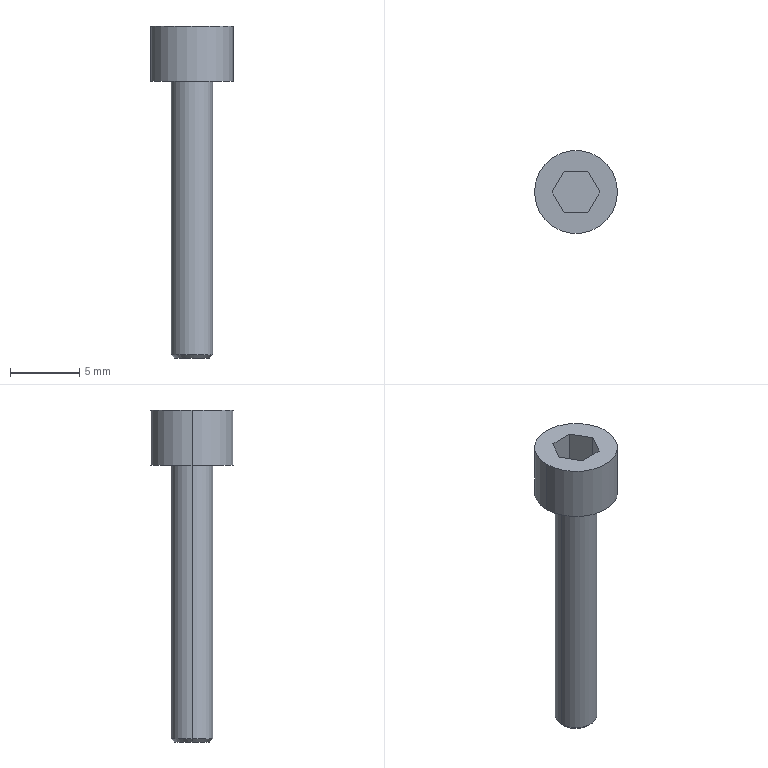Part | SolidWorks | features BaseBody 1 | 1 solid | 16 faces | box 6 x 6 x 24 mm | volume 234.705 mm3 | plane 10 | cylinder 4 | cone 2 | commonest cylinder face diameters 3 x2 6 x2
STEP:
#1=CARTESIAN_POINT('',(1.25,0.,-20.));
#2=VERTEX_POINT('',#1);
#3=CARTESIAN_POINT('',(-1.25,0.,-20.));
#4=VERTEX_POINT('',#3);
#5=CARTESIAN_POINT('',(0.,0.,-20.));
#6=DIRECTION('',(0.,0.,1.));
#7=DIRECTION('',(1.,0.,0.));
#8=AXIS2_PLACEMENT_3D('',#5,#6,#7);
#9=CIRCLE('',#8,1.25);
#10=EDGE_CURVE('',#2,#4,#9,.T.);
#11=ORIENTED_EDGE('',*,*,#10,.T.);
#12=CARTESIAN_POINT('',(-1.5,0.,-19.75));
#13=VERTEX_POINT('',#12);
#14=CARTESIAN_POINT('',(-1.375,0.,-19.875));
#15=DIRECTION('',(-0.7071,0.,0.7071));
#16=VECTOR('',#15,1000.);
#17=LINE('',#14,#16);
#18=EDGE_CURVE('',#4,#13,#17,.T.);
#19=ORIENTED_EDGE('',*,*,#18,.T.);
#20=CARTESIAN_POINT('',(1.5,0.,-19.75));
#21=VERTEX_POINT('',#20);
#22=CARTESIAN_POINT('',(0.,0.,-19.75));
#23=DIRECTION('',(0.,0.,-1.));
#24=DIRECTION('',(1.,0.,0.));
#25=AXIS2_PLACEMENT_3D('',#22,#23,#24);
#26=CIRCLE('',#25,1.5);
#27=EDGE_CURVE('',#13,#21,#26,.T.);
#28=ORIENTED_EDGE('',*,*,#27,.T.);
#29=CARTESIAN_POINT('',(1.375,0.,-19.875));
#30=DIRECTION('',(0.7071,0.,0.7071));
#31=VECTOR('',#30,1000.);
#32=LINE('',#29,#31);
#33=EDGE_CURVE('',#2,#21,#32,.T.);
#34=ORIENTED_EDGE('',*,*,#33,.F.);
#35=EDGE_LOOP('',(#11,#19,#28,#34));
#36=FACE_OUTER_BOUND('',#35,.T.);
#37=CARTESIAN_POINT('',(0.,0.,-19.875));
#38=DIRECTION('',(0.,0.,1.));
#39=DIRECTION('',(1.,0.,0.));
#40=AXIS2_PLACEMENT_3D('',#37,#38,#39);
#41=CONICAL_SURFACE('',#40,1.375,0.7854);
#42=ADVANCED_FACE('',(#36),#41,.T.);
#43=ORIENTED_EDGE('',*,*,#27,.F.);
#44=CARTESIAN_POINT('',(-1.5,0.,0.));
#45=VERTEX_POINT('',#44);
#46=CARTESIAN_POINT('',(-1.5,0.,0.));
#47=DIRECTION('',(0.,0.,1.));
#48=VECTOR('',#47,1000.);
#49=LINE('',#46,#48);
#50=EDGE_CURVE('',#13,#45,#49,.T.);
#51=ORIENTED_EDGE('',*,*,#50,.T.);
#52=CARTESIAN_POINT('',(1.5,0.,0.));
#53=VERTEX_POINT('',#52);
#54=CARTESIAN_POINT('',(0.,0.,0.));
#55=DIRECTION('',(0.,0.,1.));
#56=DIRECTION('',(1.,0.,0.));
#57=AXIS2_PLACEMENT_3D('',#54,#55,#56);
#58=CIRCLE('',#57,1.5);
#59=EDGE_CURVE('',#53,#45,#58,.T.);
#60=ORIENTED_EDGE('',*,*,#59,.F.);
#61=CARTESIAN_POINT('',(1.5,0.,0.));
#62=DIRECTION('',(0.,0.,1.));
#63=VECTOR('',#62,1000.);
#64=LINE('',#61,#63);
#65=EDGE_CURVE('',#21,#53,#64,.T.);
#66=ORIENTED_EDGE('',*,*,#65,.F.);
#67=EDGE_LOOP('',(#43,#51,#60,#66));
#68=FACE_OUTER_BOUND('',#67,.T.);
#69=CARTESIAN_POINT('',(0.,0.,0.));
#70=DIRECTION('',(0.,0.,1.));
#71=DIRECTION('',(1.,0.,0.));
#72=AXIS2_PLACEMENT_3D('',#69,#70,#71);
#73=CYLINDRICAL_SURFACE('',#72,1.5);
#74=ADVANCED_FACE('',(#68),#73,.T.);
#75=CARTESIAN_POINT('',(3.,0.,4.));
#76=VERTEX_POINT('',#75);
#77=CARTESIAN_POINT('',(-3.,0.,4.));
#78=VERTEX_POINT('',#77);
#79=CARTESIAN_POINT('',(0.,0.,4.));
#80=DIRECTION('',(0.,0.,1.));
#81=DIRECTION('',(-1.,0.,0.));
#82=AXIS2_PLACEMENT_3D('',#79,#80,#81);
#83=CIRCLE('',#82,3.);
#84=EDGE_CURVE('',#76,#78,#83,.T.);
#85=ORIENTED_EDGE('',*,*,#84,.F.);
#86=CARTESIAN_POINT('',(3.,0.,0.));
#87=VERTEX_POINT('',#86);
#88=CARTESIAN_POINT('',(3.,0.,0.));
#89=DIRECTION('',(0.,0.,-1.));
#90=VECTOR('',#89,1000.);
#91=LINE('',#88,#90);
#92=EDGE_CURVE('',#76,#87,#91,.T.);
#93=ORIENTED_EDGE('',*,*,#92,.T.);
#94=CARTESIAN_POINT('',(-3.,0.,0.));
#95=VERTEX_POINT('',#94);
#96=CARTESIAN_POINT('',(0.,0.,0.));
#97=DIRECTION('',(0.,0.,-1.));
#98=DIRECTION('',(-1.,0.,0.));
#99=AXIS2_PLACEMENT_3D('',#96,#97,#98);
#100=CIRCLE('',#99,3.);
#101=EDGE_CURVE('',#95,#87,#100,.T.);
#102=ORIENTED_EDGE('',*,*,#101,.F.);
#103=CARTESIAN_POINT('',(-3.,0.,0.));
#104=DIRECTION('',(0.,0.,-1.));
#105=VECTOR('',#104,1000.);
#106=LINE('',#103,#105);
#107=EDGE_CURVE('',#78,#95,#106,.T.);
#108=ORIENTED_EDGE('',*,*,#107,.F.);
#109=EDGE_LOOP('',(#85,#93,#102,#108));
#110=FACE_OUTER_BOUND('',#109,.T.);
#111=CARTESIAN_POINT('',(0.,0.,0.));
#112=DIRECTION('',(0.,0.,-1.));
#113=DIRECTION('',(-1.,0.,0.));
#114=AXIS2_PLACEMENT_3D('',#111,#112,#113);
#115=CYLINDRICAL_SURFACE('',#114,3.);
#116=ADVANCED_FACE('',(#110),#115,.T.);
#117=ORIENTED_EDGE('',*,*,#10,.F.);
#118=CARTESIAN_POINT('',(0.,0.,-20.));
#119=DIRECTION('',(0.,0.,1.));
#120=DIRECTION('',(1.,0.,0.));
#121=AXIS2_PLACEMENT_3D('',#118,#119,#120);
#122=CIRCLE('',#121,1.25);
#123=EDGE_CURVE('',#4,#2,#122,.T.);
#124=ORIENTED_EDGE('',*,*,#123,.F.);
#125=EDGE_LOOP('',(#117,#124));
#126=FACE_OUTER_BOUND('',#125,.T.);
#127=CARTESIAN_POINT('',(0.,0.,-20.));
#128=DIRECTION('',(0.,0.,1.));
#129=DIRECTION('',(1.,0.,0.));
#130=AXIS2_PLACEMENT_3D('',#127,#128,#129);
#131=PLANE('',#130);
#132=ADVANCED_FACE('',(#126),#131,.F.);
#133=CARTESIAN_POINT('',(1.732,0.,4.));
#134=VERTEX_POINT('',#133);
#135=CARTESIAN_POINT('',(0.866,-1.5,4.));
#136=VERTEX_POINT('',#135);
#137=CARTESIAN_POINT('',(1.516,-0.375,4.));
#138=DIRECTION('',(-0.5,-0.866,0.));
#139=VECTOR('',#138,1000.);
#140=LINE('',#137,#139);
#141=EDGE_CURVE('',#134,#136,#140,.T.);
#142=ORIENTED_EDGE('',*,*,#141,.F.);
#143=CARTESIAN_POINT('',(1.732,0.,1.5));
#144=VERTEX_POINT('',#143);
#145=CARTESIAN_POINT('',(1.732,0.,4.));
#146=DIRECTION('',(0.,0.,-1.));
#147=VECTOR('',#146,1000.);
#148=LINE('',#145,#147);
#149=EDGE_CURVE('',#134,#144,#148,.T.);
#150=ORIENTED_EDGE('',*,*,#149,.T.);
#151=CARTESIAN_POINT('',(0.866,-1.5,1.5));
#152=VERTEX_POINT('',#151);
#153=CARTESIAN_POINT('',(1.732,0.,1.5));
#154=DIRECTION('',(-0.5,-0.866,0.));
#155=VECTOR('',#154,1000.);
#156=LINE('',#153,#155);
#157=EDGE_CURVE('',#144,#152,#156,.T.);
#158=ORIENTED_EDGE('',*,*,#157,.T.);
#159=CARTESIAN_POINT('',(0.866,-1.5,4.));
#160=DIRECTION('',(0.,0.,-1.));
#161=VECTOR('',#160,1000.);
#162=LINE('',#159,#161);
#163=EDGE_CURVE('',#136,#152,#162,.T.);
#164=ORIENTED_EDGE('',*,*,#163,.F.);
#165=EDGE_LOOP('',(#142,#150,#158,#164));
#166=FACE_OUTER_BOUND('',#165,.T.);
#167=CARTESIAN_POINT('',(1.732,0.,4.));
#168=DIRECTION('',(0.866,-0.5,0.));
#169=DIRECTION('',(0.,0.,-1.));
#170=AXIS2_PLACEMENT_3D('',#167,#168,#169);
#171=PLANE('',#170);
#172=ADVANCED_FACE('',(#166),#171,.F.);
#173=CARTESIAN_POINT('',(0.866,1.5,4.));
#174=VERTEX_POINT('',#173);
#175=CARTESIAN_POINT('',(1.083,1.125,4.));
#176=DIRECTION('',(0.5,-0.866,0.));
#177=VECTOR('',#176,1000.);
#178=LINE('',#175,#177);
#179=EDGE_CURVE('',#174,#134,#178,.T.);
#180=ORIENTED_EDGE('',*,*,#179,.F.);
#181=CARTESIAN_POINT('',(0.866,1.5,1.5));
#182=VERTEX_POINT('',#181);
#183=CARTESIAN_POINT('',(0.866,1.5,4.));
#184=DIRECTION('',(0.,0.,-1.));
#185=VECTOR('',#184,1000.);
#186=LINE('',#183,#185);
#187=EDGE_CURVE('',#174,#182,#186,.T.);
#188=ORIENTED_EDGE('',*,*,#187,.T.);
#189=CARTESIAN_POINT('',(0.866,1.5,1.5));
#190=DIRECTION('',(0.5,-0.866,0.));
#191=VECTOR('',#190,1000.);
#192=LINE('',#189,#191);
#193=EDGE_CURVE('',#182,#144,#192,.T.);
#194=ORIENTED_EDGE('',*,*,#193,.T.);
#195=ORIENTED_EDGE('',*,*,#149,.F.);
#196=EDGE_LOOP('',(#180,#188,#194,#195));
#197=FACE_OUTER_BOUND('',#196,.T.);
#198=CARTESIAN_POINT('',(0.866,1.5,4.));
#199=DIRECTION('',(0.866,0.5,0.));
#200=DIRECTION('',(0.,0.,-1.));
#201=AXIS2_PLACEMENT_3D('',#198,#199,#200);
#202=PLANE('',#201);
#203=ADVANCED_FACE('',(#197),#202,.F.);
#204=CARTESIAN_POINT('',(-0.866,1.5,4.));
#205=VERTEX_POINT('',#204);
#206=CARTESIAN_POINT('',(-0.433,1.5,4.));
#207=DIRECTION('',(1.,0.,0.));
#208=VECTOR('',#207,1000.);
#209=LINE('',#206,#208);
#210=EDGE_CURVE('',#205,#174,#209,.T.);
#211=ORIENTED_EDGE('',*,*,#210,.F.);
#212=CARTESIAN_POINT('',(-0.866,1.5,1.5));
#213=VERTEX_POINT('',#212);
#214=CARTESIAN_POINT('',(-0.866,1.5,4.));
#215=DIRECTION('',(0.,0.,-1.));
#216=VECTOR('',#215,1000.);
#217=LINE('',#214,#216);
#218=EDGE_CURVE('',#205,#213,#217,.T.);
#219=ORIENTED_EDGE('',*,*,#218,.T.);
#220=CARTESIAN_POINT('',(-0.866,1.5,1.5));
#221=DIRECTION('',(1.,0.,0.));
#222=VECTOR('',#221,1000.);
#223=LINE('',#220,#222);
#224=EDGE_CURVE('',#213,#182,#223,.T.);
#225=ORIENTED_EDGE('',*,*,#224,.T.);
#226=ORIENTED_EDGE('',*,*,#187,.F.);
#227=EDGE_LOOP('',(#211,#219,#225,#226));
#228=FACE_OUTER_BOUND('',#227,.T.);
#229=CARTESIAN_POINT('',(-0.866,1.5,4.));
#230=DIRECTION('',(0.,1.,0.));
#231=DIRECTION('',(1.,0.,0.));
#232=AXIS2_PLACEMENT_3D('',#229,#230,#231);
#233=PLANE('',#232);
#234=ADVANCED_FACE('',(#228),#233,.F.);
#235=CARTESIAN_POINT('',(-1.732,0.,4.));
#236=VERTEX_POINT('',#235);
#237=CARTESIAN_POINT('',(-1.516,0.375,4.));
#238=DIRECTION('',(0.5,0.866,0.));
#239=VECTOR('',#238,1000.);
#240=LINE('',#237,#239);
#241=EDGE_CURVE('',#236,#205,#240,.T.);
#242=ORIENTED_EDGE('',*,*,#241,.F.);
#243=CARTESIAN_POINT('',(-1.732,0.,1.5));
#244=VERTEX_POINT('',#243);
#245=CARTESIAN_POINT('',(-1.732,0.,4.));
#246=DIRECTION('',(0.,0.,-1.));
#247=VECTOR('',#246,1000.);
#248=LINE('',#245,#247);
#249=EDGE_CURVE('',#236,#244,#248,.T.);
#250=ORIENTED_EDGE('',*,*,#249,.T.);
#251=CARTESIAN_POINT('',(-1.732,0.,1.5));
#252=DIRECTION('',(0.5,0.866,0.));
#253=VECTOR('',#252,1000.);
#254=LINE('',#251,#253);
#255=EDGE_CURVE('',#244,#213,#254,.T.);
#256=ORIENTED_EDGE('',*,*,#255,.T.);
#257=ORIENTED_EDGE('',*,*,#218,.F.);
#258=EDGE_LOOP('',(#242,#250,#256,#257));
#259=FACE_OUTER_BOUND('',#258,.T.);
#260=CARTESIAN_POINT('',(-1.732,0.,4.));
#261=DIRECTION('',(-0.866,0.5,0.));
#262=DIRECTION('',(0.,0.,1.));
#263=AXIS2_PLACEMENT_3D('',#260,#261,#262);
#264=PLANE('',#263);
#265=ADVANCED_FACE('',(#259),#264,.F.);
#266=CARTESIAN_POINT('',(-0.866,-1.5,4.));
#267=VERTEX_POINT('',#266);
#268=CARTESIAN_POINT('',(-1.083,-1.125,4.));
#269=DIRECTION('',(-0.5,0.866,0.));
#270=VECTOR('',#269,1000.);
#271=LINE('',#268,#270);
#272=EDGE_CURVE('',#267,#236,#271,.T.);
#273=ORIENTED_EDGE('',*,*,#272,.F.);
#274=CARTESIAN_POINT('',(-0.866,-1.5,1.5));
#275=VERTEX_POINT('',#274);
#276=CARTESIAN_POINT('',(-0.866,-1.5,4.));
#277=DIRECTION('',(0.,0.,-1.));
#278=VECTOR('',#277,1000.);
#279=LINE('',#276,#278);
#280=EDGE_CURVE('',#267,#275,#279,.T.);
#281=ORIENTED_EDGE('',*,*,#280,.T.);
#282=CARTESIAN_POINT('',(-0.866,-1.5,1.5));
#283=DIRECTION('',(-0.5,0.866,0.));
#284=VECTOR('',#283,1000.);
#285=LINE('',#282,#284);
#286=EDGE_CURVE('',#275,#244,#285,.T.);
#287=ORIENTED_EDGE('',*,*,#286,.T.);
#288=ORIENTED_EDGE('',*,*,#249,.F.);
#289=EDGE_LOOP('',(#273,#281,#287,#288));
#290=FACE_OUTER_BOUND('',#289,.T.);
#291=CARTESIAN_POINT('',(-0.866,-1.5,4.));
#292=DIRECTION('',(-0.866,-0.5,0.));
#293=DIRECTION('',(-0.5,0.866,0.));
#294=AXIS2_PLACEMENT_3D('',#291,#292,#293);
#295=PLANE('',#294);
#296=ADVANCED_FACE('',(#290),#295,.F.);
#297=CARTESIAN_POINT('',(0.433,-1.5,4.));
#298=DIRECTION('',(-1.,0.,0.));
#299=VECTOR('',#298,1000.);
#300=LINE('',#297,#299);
#301=EDGE_CURVE('',#136,#267,#300,.T.);
#302=ORIENTED_EDGE('',*,*,#301,.F.);
#303=ORIENTED_EDGE('',*,*,#163,.T.);
#304=CARTESIAN_POINT('',(0.866,-1.5,1.5));
#305=DIRECTION('',(-1.,0.,0.));
#306=VECTOR('',#305,1000.);
#307=LINE('',#304,#306);
#308=EDGE_CURVE('',#152,#275,#307,.T.);
#309=ORIENTED_EDGE('',*,*,#308,.T.);
#310=ORIENTED_EDGE('',*,*,#280,.F.);
#311=EDGE_LOOP('',(#302,#303,#309,#310));
#312=FACE_OUTER_BOUND('',#311,.T.);
#313=CARTESIAN_POINT('',(0.866,-1.5,4.));
#314=DIRECTION('',(0.,-1.,0.));
#315=DIRECTION('',(-1.,0.,0.));
#316=AXIS2_PLACEMENT_3D('',#313,#314,#315);
#317=PLANE('',#316);
#318=ADVANCED_FACE('',(#312),#317,.F.);
#319=ORIENTED_EDGE('',*,*,#308,.F.);
#320=ORIENTED_EDGE('',*,*,#157,.F.);
#321=ORIENTED_EDGE('',*,*,#193,.F.);
#322=ORIENTED_EDGE('',*,*,#224,.F.);
#323=ORIENTED_EDGE('',*,*,#255,.F.);
#324=ORIENTED_EDGE('',*,*,#286,.F.);
#325=EDGE_LOOP('',(#319,#320,#321,#322,#323,#324));
#326=FACE_OUTER_BOUND('',#325,.T.);
#327=CARTESIAN_POINT('',(0.,0.,1.5));
#328=DIRECTION('',(0.,0.,-1.));
#329=DIRECTION('',(0.,-1.,0.));
#330=AXIS2_PLACEMENT_3D('',#327,#328,#329);
#331=PLANE('',#330);
#332=ADVANCED_FACE('',(#326),#331,.F.);
#333=ORIENTED_EDGE('',*,*,#59,.T.);
#334=CARTESIAN_POINT('',(0.,0.,0.));
#335=DIRECTION('',(0.,0.,1.));
#336=DIRECTION('',(1.,0.,0.));
#337=AXIS2_PLACEMENT_3D('',#334,#335,#336);
#338=CIRCLE('',#337,1.5);
#339=EDGE_CURVE('',#45,#53,#338,.T.);
#340=ORIENTED_EDGE('',*,*,#339,.T.);
#341=EDGE_LOOP('',(#333,#340));
#342=FACE_BOUND('',#341,.T.);
#343=ORIENTED_EDGE('',*,*,#101,.T.);
#344=CARTESIAN_POINT('',(0.,0.,0.));
#345=DIRECTION('',(0.,0.,-1.));
#346=DIRECTION('',(-1.,0.,0.));
#347=AXIS2_PLACEMENT_3D('',#344,#345,#346);
#348=CIRCLE('',#347,3.);
#349=EDGE_CURVE('',#87,#95,#348,.T.);
#350=ORIENTED_EDGE('',*,*,#349,.T.);
#351=EDGE_LOOP('',(#343,#350));
#352=FACE_OUTER_BOUND('',#351,.T.);
#353=CARTESIAN_POINT('',(0.,0.,0.));
#354=DIRECTION('',(0.,0.,1.));
#355=DIRECTION('',(1.,0.,0.));
#356=AXIS2_PLACEMENT_3D('',#353,#354,#355);
#357=PLANE('',#356);
#358=ADVANCED_FACE('',(#342,#352),#357,.F.);
#359=ORIENTED_EDGE('',*,*,#141,.T.);
#360=ORIENTED_EDGE('',*,*,#301,.T.);
#361=ORIENTED_EDGE('',*,*,#272,.T.);
#362=ORIENTED_EDGE('',*,*,#241,.T.);
#363=ORIENTED_EDGE('',*,*,#210,.T.);
#364=ORIENTED_EDGE('',*,*,#179,.T.);
#365=EDGE_LOOP('',(#359,#360,#361,#362,#363,#364));
#366=FACE_BOUND('',#365,.T.);
#367=CARTESIAN_POINT('',(0.,0.,4.));
#368=DIRECTION('',(0.,0.,1.));
#369=DIRECTION('',(-1.,0.,0.));
#370=AXIS2_PLACEMENT_3D('',#367,#368,#369);
#371=CIRCLE('',#370,3.);
#372=EDGE_CURVE('',#78,#76,#371,.T.);
#373=ORIENTED_EDGE('',*,*,#372,.T.);
#374=ORIENTED_EDGE('',*,*,#84,.T.);
#375=EDGE_LOOP('',(#373,#374));
#376=FACE_OUTER_BOUND('',#375,.T.);
#377=CARTESIAN_POINT('',(0.,0.,4.));
#378=DIRECTION('',(0.,0.,1.));
#379=DIRECTION('',(1.,0.,0.));
#380=AXIS2_PLACEMENT_3D('',#377,#378,#379);
#381=PLANE('',#380);
#382=ADVANCED_FACE('',(#366,#376),#381,.T.);
#383=ORIENTED_EDGE('',*,*,#92,.F.);
#384=ORIENTED_EDGE('',*,*,#372,.F.);
#385=ORIENTED_EDGE('',*,*,#107,.T.);
#386=ORIENTED_EDGE('',*,*,#349,.F.);
#387=EDGE_LOOP('',(#383,#384,#385,#386));
#388=FACE_OUTER_BOUND('',#387,.T.);
#389=CARTESIAN_POINT('',(0.,0.,0.));
#390=DIRECTION('',(0.,0.,-1.));
#391=DIRECTION('',(-1.,0.,0.));
#392=AXIS2_PLACEMENT_3D('',#389,#390,#391);
#393=CYLINDRICAL_SURFACE('',#392,3.);
#394=ADVANCED_FACE('',(#388),#393,.T.);
#395=ORIENTED_EDGE('',*,*,#50,.F.);
#396=CARTESIAN_POINT('',(0.,0.,-19.75));
#397=DIRECTION('',(0.,0.,-1.));
#398=DIRECTION('',(1.,0.,0.));
#399=AXIS2_PLACEMENT_3D('',#396,#397,#398);
#400=CIRCLE('',#399,1.5);
#401=EDGE_CURVE('',#21,#13,#400,.T.);
#402=ORIENTED_EDGE('',*,*,#401,.F.);
#403=ORIENTED_EDGE('',*,*,#65,.T.);
#404=ORIENTED_EDGE('',*,*,#339,.F.);
#405=EDGE_LOOP('',(#395,#402,#403,#404));
#406=FACE_OUTER_BOUND('',#405,.T.);
#407=CARTESIAN_POINT('',(0.,0.,0.));
#408=DIRECTION('',(0.,0.,1.));
#409=DIRECTION('',(1.,0.,0.));
#410=AXIS2_PLACEMENT_3D('',#407,#408,#409);
#411=CYLINDRICAL_SURFACE('',#410,1.5);
#412=ADVANCED_FACE('',(#406),#411,.T.);
#413=ORIENTED_EDGE('',*,*,#18,.F.);
#414=ORIENTED_EDGE('',*,*,#123,.T.);
#415=ORIENTED_EDGE('',*,*,#33,.T.);
#416=ORIENTED_EDGE('',*,*,#401,.T.);
#417=EDGE_LOOP('',(#413,#414,#415,#416));
#418=FACE_OUTER_BOUND('',#417,.T.);
#419=CARTESIAN_POINT('',(0.,0.,-19.875));
#420=DIRECTION('',(0.,0.,1.));
#421=DIRECTION('',(1.,0.,0.));
#422=AXIS2_PLACEMENT_3D('',#419,#420,#421);
#423=CONICAL_SURFACE('',#422,1.375,0.7854);
#424=ADVANCED_FACE('',(#418),#423,.T.);
#425=CLOSED_SHELL('',(#42,#74,#116,#132,#172,#203,#234,#265,#296,#318,#332,#358,#382,#394,#412,#424));
#426=MANIFOLD_SOLID_BREP('',#425);
#427=CARTESIAN_POINT('',(0.,0.,0.));
#428=DIRECTION('',(0.,0.,1.));
#429=DIRECTION('',(1.,0.,0.));
#430=AXIS2_PLACEMENT_3D('',#427,#428,#429);
#431=(LENGTH_UNIT()NAMED_UNIT(*)SI_UNIT(.MILLI.,.METRE.));
#432=UNCERTAINTY_MEASURE_WITH_UNIT(LENGTH_MEASURE(0.00001),#431,'','');
#433=(NAMED_UNIT(*)PLANE_ANGLE_UNIT()SI_UNIT($,.RADIAN.));
#434=(NAMED_UNIT(*)SI_UNIT($,.STERADIAN.)SOLID_ANGLE_UNIT());
#435=(GEOMETRIC_REPRESENTATION_CONTEXT(3)GLOBAL_UNCERTAINTY_ASSIGNED_CONTEXT((#432))GLOBAL_UNIT_ASSIGNED_CONTEXT((#431,#433,#434))REPRESENTATION_CONTEXT('',''));
#436=ADVANCED_BREP_SHAPE_REPRESENTATION('',(#426,#430),#435);